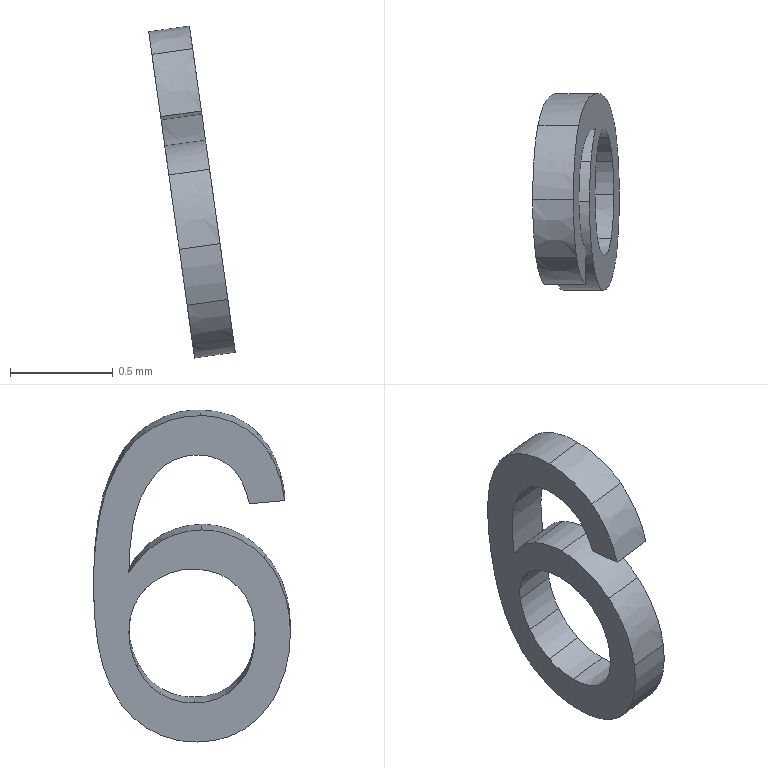Part | Creo | 1 solid | 30 faces | box 0.4214 x 0.9586 x 1.617 mm | volume 0.1424 mm3 | other 28 | plane 2